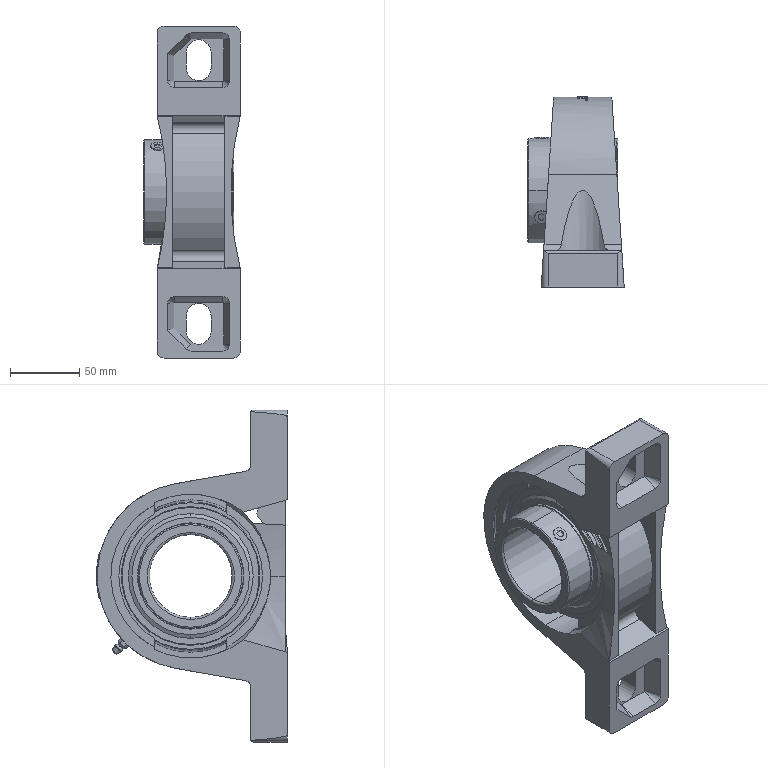Part | SolidWorks | features AEMSimFeature 1 | 13 solids | 479 faces | box 69.7 x 138 x 240 mm | volume 620717 mm3 | plane 156 | cylinder 145 | cone 96 | torus 50 | sphere 32 | commonest cylinder face diameters 0.242 x14 0.416 x14 10 x14 75.64 x14 0.769 x13 0.236 x10